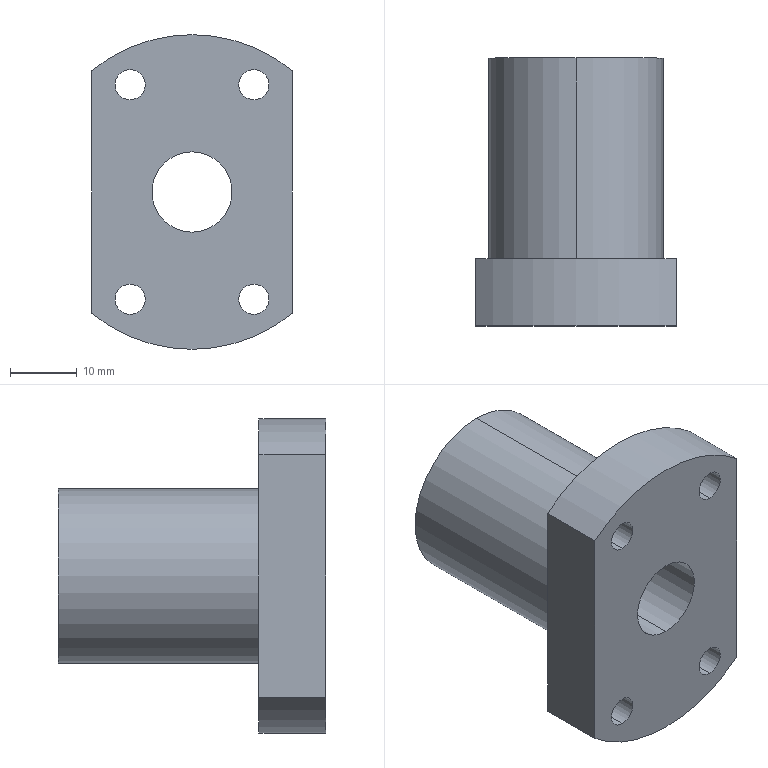Part | NX | features BREP 1 | 1 solid | 20 faces | box 30 x 40 x 47 mm | volume 23841 mm3 | cylinder 15 | plane 5 | commonest cylinder face diameters 4.5 x8 47 x3 12 x2 26 x2
STEP:
#1=CARTESIAN_POINT('',(15.,10.,-18.09));
#2=VERTEX_POINT('',#1);
#3=CARTESIAN_POINT('',(15.,10.,18.09));
#4=VERTEX_POINT('',#3);
#5=CARTESIAN_POINT('',(15.,10.,0.));
#6=DIRECTION('',(0.,0.,1.));
#7=VECTOR('',#6,1000.);
#8=LINE('',#5,#7);
#9=EDGE_CURVE('',#2,#4,#8,.T.);
#10=ORIENTED_EDGE('',*,*,#9,.T.);
#11=CARTESIAN_POINT('',(15.,0.,18.09));
#12=VERTEX_POINT('',#11);
#13=CARTESIAN_POINT('',(15.,40.,18.09));
#14=DIRECTION('',(0.,-1.,0.));
#15=VECTOR('',#14,1000.);
#16=LINE('',#13,#15);
#17=EDGE_CURVE('',#4,#12,#16,.T.);
#18=ORIENTED_EDGE('',*,*,#17,.T.);
#19=CARTESIAN_POINT('',(15.,0.,-18.09));
#20=VERTEX_POINT('',#19);
#21=CARTESIAN_POINT('',(15.,0.,-18.09));
#22=DIRECTION('',(0.,0.,1.));
#23=VECTOR('',#22,1000.);
#24=LINE('',#21,#23);
#25=EDGE_CURVE('',#20,#12,#24,.T.);
#26=ORIENTED_EDGE('',*,*,#25,.F.);
#27=CARTESIAN_POINT('',(15.,40.,-18.09));
#28=DIRECTION('',(0.,-1.,0.));
#29=VECTOR('',#28,1000.);
#30=LINE('',#27,#29);
#31=EDGE_CURVE('',#2,#20,#30,.T.);
#32=ORIENTED_EDGE('',*,*,#31,.F.);
#33=EDGE_LOOP('',(#10,#18,#26,#32));
#34=FACE_BOUND('',#33,.T.);
#35=CARTESIAN_POINT('',(15.,40.,-18.09));
#36=DIRECTION('',(1.,0.,0.));
#37=DIRECTION('',(0.,0.,-1.));
#38=AXIS2_PLACEMENT_3D('',#35,#36,#37);
#39=PLANE('',#38);
#40=ADVANCED_FACE('',(#34),#39,.T.);
#41=CARTESIAN_POINT('',(-15.,10.,18.09));
#42=VERTEX_POINT('',#41);
#43=CARTESIAN_POINT('',(-15.,10.,-18.09));
#44=VERTEX_POINT('',#43);
#45=CARTESIAN_POINT('',(-15.,10.,0.));
#46=DIRECTION('',(0.,0.,-1.));
#47=VECTOR('',#46,1000.);
#48=LINE('',#45,#47);
#49=EDGE_CURVE('',#42,#44,#48,.T.);
#50=ORIENTED_EDGE('',*,*,#49,.T.);
#51=CARTESIAN_POINT('',(-15.,0.,-18.09));
#52=VERTEX_POINT('',#51);
#53=CARTESIAN_POINT('',(-15.,40.,-18.09));
#54=DIRECTION('',(0.,-1.,0.));
#55=VECTOR('',#54,1000.);
#56=LINE('',#53,#55);
#57=EDGE_CURVE('',#44,#52,#56,.T.);
#58=ORIENTED_EDGE('',*,*,#57,.T.);
#59=CARTESIAN_POINT('',(-15.,0.,18.09));
#60=VERTEX_POINT('',#59);
#61=CARTESIAN_POINT('',(-15.,0.,-18.09));
#62=DIRECTION('',(0.,0.,-1.));
#63=VECTOR('',#62,1000.);
#64=LINE('',#61,#63);
#65=EDGE_CURVE('',#60,#52,#64,.T.);
#66=ORIENTED_EDGE('',*,*,#65,.F.);
#67=CARTESIAN_POINT('',(-15.,40.,18.09));
#68=DIRECTION('',(0.,-1.,0.));
#69=VECTOR('',#68,1000.);
#70=LINE('',#67,#69);
#71=EDGE_CURVE('',#42,#60,#70,.T.);
#72=ORIENTED_EDGE('',*,*,#71,.F.);
#73=EDGE_LOOP('',(#50,#58,#66,#72));
#74=FACE_BOUND('',#73,.T.);
#75=CARTESIAN_POINT('',(-15.,40.,-18.09));
#76=DIRECTION('',(-1.,0.,0.));
#77=DIRECTION('',(0.,0.,1.));
#78=AXIS2_PLACEMENT_3D('',#75,#76,#77);
#79=PLANE('',#78);
#80=ADVANCED_FACE('',(#74),#79,.T.);
#81=CARTESIAN_POINT('',(9.25,10.,18.271));
#82=VERTEX_POINT('',#81);
#83=CARTESIAN_POINT('',(9.25,0.,18.271));
#84=VERTEX_POINT('',#83);
#85=CARTESIAN_POINT('',(9.25,40.,18.271));
#86=DIRECTION('',(0.,-1.,0.));
#87=VECTOR('',#86,1000.);
#88=LINE('',#85,#87);
#89=EDGE_CURVE('',#82,#84,#88,.T.);
#90=ORIENTED_EDGE('',*,*,#89,.F.);
#91=CARTESIAN_POINT('',(9.25,10.,13.771));
#92=VERTEX_POINT('',#91);
#93=CARTESIAN_POINT('',(9.25,10.,16.021));
#94=DIRECTION('',(0.,-1.,0.));
#95=DIRECTION('',(0.,0.,-1.));
#96=AXIS2_PLACEMENT_3D('',#93,#94,#95);
#97=CIRCLE('',#96,2.25);
#98=EDGE_CURVE('',#92,#82,#97,.T.);
#99=ORIENTED_EDGE('',*,*,#98,.F.);
#100=CARTESIAN_POINT('',(9.25,0.,13.771));
#101=VERTEX_POINT('',#100);
#102=CARTESIAN_POINT('',(9.25,40.,13.771));
#103=DIRECTION('',(0.,-1.,0.));
#104=VECTOR('',#103,1000.);
#105=LINE('',#102,#104);
#106=EDGE_CURVE('',#92,#101,#105,.T.);
#107=ORIENTED_EDGE('',*,*,#106,.T.);
#108=CARTESIAN_POINT('',(9.25,0.,16.021));
#109=DIRECTION('',(0.,-1.,0.));
#110=DIRECTION('',(0.,0.,1.));
#111=AXIS2_PLACEMENT_3D('',#108,#109,#110);
#112=CIRCLE('',#111,2.25);
#113=EDGE_CURVE('',#101,#84,#112,.T.);
#114=ORIENTED_EDGE('',*,*,#113,.T.);
#115=EDGE_LOOP('',(#90,#99,#107,#114));
#116=FACE_BOUND('',#115,.T.);
#117=CARTESIAN_POINT('',(9.25,40.,16.021));
#118=DIRECTION('',(0.,-1.,0.));
#119=DIRECTION('',(0.,0.,-1.));
#120=AXIS2_PLACEMENT_3D('',#117,#118,#119);
#121=CYLINDRICAL_SURFACE('',#120,2.25);
#122=ADVANCED_FACE('',(#116),#121,.F.);
#123=CARTESIAN_POINT('',(9.25,10.,-13.771));
#124=VERTEX_POINT('',#123);
#125=CARTESIAN_POINT('',(9.25,0.,-13.771));
#126=VERTEX_POINT('',#125);
#127=CARTESIAN_POINT('',(9.25,40.,-13.771));
#128=DIRECTION('',(0.,-1.,0.));
#129=VECTOR('',#128,1000.);
#130=LINE('',#127,#129);
#131=EDGE_CURVE('',#124,#126,#130,.T.);
#132=ORIENTED_EDGE('',*,*,#131,.F.);
#133=CARTESIAN_POINT('',(9.25,10.,-18.271));
#134=VERTEX_POINT('',#133);
#135=CARTESIAN_POINT('',(9.25,10.,-16.021));
#136=DIRECTION('',(0.,-1.,0.));
#137=DIRECTION('',(0.,0.,-1.));
#138=AXIS2_PLACEMENT_3D('',#135,#136,#137);
#139=CIRCLE('',#138,2.25);
#140=EDGE_CURVE('',#134,#124,#139,.T.);
#141=ORIENTED_EDGE('',*,*,#140,.F.);
#142=CARTESIAN_POINT('',(9.25,0.,-18.271));
#143=VERTEX_POINT('',#142);
#144=CARTESIAN_POINT('',(9.25,40.,-18.271));
#145=DIRECTION('',(0.,-1.,0.));
#146=VECTOR('',#145,1000.);
#147=LINE('',#144,#146);
#148=EDGE_CURVE('',#134,#143,#147,.T.);
#149=ORIENTED_EDGE('',*,*,#148,.T.);
#150=CARTESIAN_POINT('',(9.25,0.,-16.021));
#151=DIRECTION('',(0.,-1.,0.));
#152=DIRECTION('',(0.,0.,-1.));
#153=AXIS2_PLACEMENT_3D('',#150,#151,#152);
#154=CIRCLE('',#153,2.25);
#155=EDGE_CURVE('',#143,#126,#154,.T.);
#156=ORIENTED_EDGE('',*,*,#155,.T.);
#157=EDGE_LOOP('',(#132,#141,#149,#156));
#158=FACE_BOUND('',#157,.T.);
#159=CARTESIAN_POINT('',(9.25,40.,-16.021));
#160=DIRECTION('',(0.,-1.,0.));
#161=DIRECTION('',(0.,0.,-1.));
#162=AXIS2_PLACEMENT_3D('',#159,#160,#161);
#163=CYLINDRICAL_SURFACE('',#162,2.25);
#164=ADVANCED_FACE('',(#158),#163,.F.);
#165=CARTESIAN_POINT('',(-9.25,10.,-13.771));
#166=VERTEX_POINT('',#165);
#167=CARTESIAN_POINT('',(-9.25,0.,-13.771));
#168=VERTEX_POINT('',#167);
#169=CARTESIAN_POINT('',(-9.25,40.,-13.771));
#170=DIRECTION('',(0.,-1.,0.));
#171=VECTOR('',#170,1000.);
#172=LINE('',#169,#171);
#173=EDGE_CURVE('',#166,#168,#172,.T.);
#174=ORIENTED_EDGE('',*,*,#173,.F.);
#175=CARTESIAN_POINT('',(-9.25,10.,-18.271));
#176=VERTEX_POINT('',#175);
#177=CARTESIAN_POINT('',(-9.25,10.,-16.021));
#178=DIRECTION('',(0.,-1.,0.));
#179=DIRECTION('',(0.,0.,-1.));
#180=AXIS2_PLACEMENT_3D('',#177,#178,#179);
#181=CIRCLE('',#180,2.25);
#182=EDGE_CURVE('',#176,#166,#181,.T.);
#183=ORIENTED_EDGE('',*,*,#182,.F.);
#184=CARTESIAN_POINT('',(-9.25,0.,-18.271));
#185=VERTEX_POINT('',#184);
#186=CARTESIAN_POINT('',(-9.25,40.,-18.271));
#187=DIRECTION('',(0.,-1.,0.));
#188=VECTOR('',#187,1000.);
#189=LINE('',#186,#188);
#190=EDGE_CURVE('',#176,#185,#189,.T.);
#191=ORIENTED_EDGE('',*,*,#190,.T.);
#192=CARTESIAN_POINT('',(-9.25,0.,-16.021));
#193=DIRECTION('',(0.,-1.,0.));
#194=DIRECTION('',(0.,0.,1.));
#195=AXIS2_PLACEMENT_3D('',#192,#193,#194);
#196=CIRCLE('',#195,2.25);
#197=EDGE_CURVE('',#185,#168,#196,.T.);
#198=ORIENTED_EDGE('',*,*,#197,.T.);
#199=EDGE_LOOP('',(#174,#183,#191,#198));
#200=FACE_BOUND('',#199,.T.);
#201=CARTESIAN_POINT('',(-9.25,40.,-16.021));
#202=DIRECTION('',(0.,-1.,0.));
#203=DIRECTION('',(0.,0.,-1.));
#204=AXIS2_PLACEMENT_3D('',#201,#202,#203);
#205=CYLINDRICAL_SURFACE('',#204,2.25);
#206=ADVANCED_FACE('',(#200),#205,.F.);
#207=CARTESIAN_POINT('',(-9.25,10.,18.271));
#208=VERTEX_POINT('',#207);
#209=CARTESIAN_POINT('',(-9.25,0.,18.271));
#210=VERTEX_POINT('',#209);
#211=CARTESIAN_POINT('',(-9.25,40.,18.271));
#212=DIRECTION('',(0.,-1.,0.));
#213=VECTOR('',#212,1000.);
#214=LINE('',#211,#213);
#215=EDGE_CURVE('',#208,#210,#214,.T.);
#216=ORIENTED_EDGE('',*,*,#215,.F.);
#217=CARTESIAN_POINT('',(-9.25,10.,13.771));
#218=VERTEX_POINT('',#217);
#219=CARTESIAN_POINT('',(-9.25,10.,16.021));
#220=DIRECTION('',(0.,-1.,0.));
#221=DIRECTION('',(0.,0.,-1.));
#222=AXIS2_PLACEMENT_3D('',#219,#220,#221);
#223=CIRCLE('',#222,2.25);
#224=EDGE_CURVE('',#218,#208,#223,.T.);
#225=ORIENTED_EDGE('',*,*,#224,.F.);
#226=CARTESIAN_POINT('',(-9.25,0.,13.771));
#227=VERTEX_POINT('',#226);
#228=CARTESIAN_POINT('',(-9.25,40.,13.771));
#229=DIRECTION('',(0.,-1.,0.));
#230=VECTOR('',#229,1000.);
#231=LINE('',#228,#230);
#232=EDGE_CURVE('',#218,#227,#231,.T.);
#233=ORIENTED_EDGE('',*,*,#232,.T.);
#234=CARTESIAN_POINT('',(-9.25,0.,16.021));
#235=DIRECTION('',(0.,-1.,0.));
#236=DIRECTION('',(0.,0.,-1.));
#237=AXIS2_PLACEMENT_3D('',#234,#235,#236);
#238=CIRCLE('',#237,2.25);
#239=EDGE_CURVE('',#227,#210,#238,.T.);
#240=ORIENTED_EDGE('',*,*,#239,.T.);
#241=EDGE_LOOP('',(#216,#225,#233,#240));
#242=FACE_BOUND('',#241,.T.);
#243=CARTESIAN_POINT('',(-9.25,40.,16.021));
#244=DIRECTION('',(0.,-1.,0.));
#245=DIRECTION('',(0.,0.,-1.));
#246=AXIS2_PLACEMENT_3D('',#243,#244,#245);
#247=CYLINDRICAL_SURFACE('',#246,2.25);
#248=ADVANCED_FACE('',(#242),#247,.F.);
#249=CARTESIAN_POINT('',(0.,40.,-6.));
#250=VERTEX_POINT('',#249);
#251=CARTESIAN_POINT('',(0.,40.,6.));
#252=VERTEX_POINT('',#251);
#253=CARTESIAN_POINT('',(0.,40.,0.));
#254=DIRECTION('',(0.,-1.,0.));
#255=DIRECTION('',(0.,0.,-1.));
#256=AXIS2_PLACEMENT_3D('',#253,#254,#255);
#257=CIRCLE('',#256,6.);
#258=EDGE_CURVE('',#250,#252,#257,.T.);
#259=ORIENTED_EDGE('',*,*,#258,.T.);
#260=CARTESIAN_POINT('',(0.,40.,0.));
#261=DIRECTION('',(0.,-1.,0.));
#262=DIRECTION('',(0.,0.,-1.));
#263=AXIS2_PLACEMENT_3D('',#260,#261,#262);
#264=CIRCLE('',#263,6.);
#265=EDGE_CURVE('',#252,#250,#264,.T.);
#266=ORIENTED_EDGE('',*,*,#265,.T.);
#267=EDGE_LOOP('',(#259,#266));
#268=FACE_BOUND('',#267,.T.);
#269=CARTESIAN_POINT('',(0.,40.,-13.));
#270=VERTEX_POINT('',#269);
#271=CARTESIAN_POINT('',(0.,40.,13.));
#272=VERTEX_POINT('',#271);
#273=CARTESIAN_POINT('',(0.,40.,0.));
#274=DIRECTION('',(0.,-1.,0.));
#275=DIRECTION('',(0.,0.,-1.));
#276=AXIS2_PLACEMENT_3D('',#273,#274,#275);
#277=CIRCLE('',#276,13.);
#278=EDGE_CURVE('',#270,#272,#277,.T.);
#279=ORIENTED_EDGE('',*,*,#278,.F.);
#280=CARTESIAN_POINT('',(0.,40.,0.));
#281=DIRECTION('',(0.,-1.,0.));
#282=DIRECTION('',(0.,0.,-1.));
#283=AXIS2_PLACEMENT_3D('',#280,#281,#282);
#284=CIRCLE('',#283,13.);
#285=EDGE_CURVE('',#272,#270,#284,.T.);
#286=ORIENTED_EDGE('',*,*,#285,.F.);
#287=EDGE_LOOP('',(#279,#286));
#288=FACE_BOUND('',#287,.T.);
#289=CARTESIAN_POINT('',(-13.,40.,0.));
#290=DIRECTION('',(0.,-1.,0.));
#291=DIRECTION('',(0.,0.,-1.));
#292=AXIS2_PLACEMENT_3D('',#289,#290,#291);
#293=PLANE('',#292);
#294=ADVANCED_FACE('',(#268,#288),#293,.F.);
#295=CARTESIAN_POINT('',(0.,10.,13.));
#296=VERTEX_POINT('',#295);
#297=CARTESIAN_POINT('',(0.,0.,13.));
#298=DIRECTION('',(0.,-1.,0.));
#299=VECTOR('',#298,1000.);
#300=LINE('',#297,#299);
#301=EDGE_CURVE('',#272,#296,#300,.T.);
#302=ORIENTED_EDGE('',*,*,#301,.F.);
#303=ORIENTED_EDGE('',*,*,#285,.T.);
#304=CARTESIAN_POINT('',(0.,10.,-13.));
#305=VERTEX_POINT('',#304);
#306=CARTESIAN_POINT('',(0.,0.,-13.));
#307=DIRECTION('',(0.,-1.,0.));
#308=VECTOR('',#307,1000.);
#309=LINE('',#306,#308);
#310=EDGE_CURVE('',#270,#305,#309,.T.);
#311=ORIENTED_EDGE('',*,*,#310,.T.);
#312=CARTESIAN_POINT('',(0.,10.,0.));
#313=DIRECTION('',(0.,-1.,0.));
#314=DIRECTION('',(0.,0.,-1.));
#315=AXIS2_PLACEMENT_3D('',#312,#313,#314);
#316=CIRCLE('',#315,13.);
#317=EDGE_CURVE('',#296,#305,#316,.T.);
#318=ORIENTED_EDGE('',*,*,#317,.F.);
#319=EDGE_LOOP('',(#302,#303,#311,#318));
#320=FACE_BOUND('',#319,.T.);
#321=CARTESIAN_POINT('',(0.,0.,0.));
#322=DIRECTION('',(0.,-1.,0.));
#323=DIRECTION('',(0.,0.,-1.));
#324=AXIS2_PLACEMENT_3D('',#321,#322,#323);
#325=CYLINDRICAL_SURFACE('',#324,13.);
#326=ADVANCED_FACE('',(#320),#325,.T.);
#327=CARTESIAN_POINT('',(0.,0.,6.));
#328=VERTEX_POINT('',#327);
#329=CARTESIAN_POINT('',(0.,0.,6.));
#330=DIRECTION('',(0.,-1.,0.));
#331=VECTOR('',#330,1000.);
#332=LINE('',#329,#331);
#333=EDGE_CURVE('',#252,#328,#332,.T.);
#334=ORIENTED_EDGE('',*,*,#333,.F.);
#335=ORIENTED_EDGE('',*,*,#258,.F.);
#336=CARTESIAN_POINT('',(0.,0.,-6.));
#337=VERTEX_POINT('',#336);
#338=CARTESIAN_POINT('',(0.,0.,-6.));
#339=DIRECTION('',(0.,-1.,0.));
#340=VECTOR('',#339,1000.);
#341=LINE('',#338,#340);
#342=EDGE_CURVE('',#250,#337,#341,.T.);
#343=ORIENTED_EDGE('',*,*,#342,.T.);
#344=CARTESIAN_POINT('',(0.,0.,0.));
#345=DIRECTION('',(0.,-1.,0.));
#346=DIRECTION('',(0.,0.,-1.));
#347=AXIS2_PLACEMENT_3D('',#344,#345,#346);
#348=CIRCLE('',#347,6.);
#349=EDGE_CURVE('',#337,#328,#348,.T.);
#350=ORIENTED_EDGE('',*,*,#349,.T.);
#351=EDGE_LOOP('',(#334,#335,#343,#350));
#352=FACE_BOUND('',#351,.T.);
#353=CARTESIAN_POINT('',(0.,0.,0.));
#354=DIRECTION('',(0.,-1.,0.));
#355=DIRECTION('',(0.,0.,-1.));
#356=AXIS2_PLACEMENT_3D('',#353,#354,#355);
#357=CYLINDRICAL_SURFACE('',#356,6.);
#358=ADVANCED_FACE('',(#352),#357,.F.);
#359=ORIENTED_EDGE('',*,*,#9,.F.);
#360=CARTESIAN_POINT('',(0.,10.,-23.5));
#361=VERTEX_POINT('',#360);
#362=CARTESIAN_POINT('',(0.,10.,0.));
#363=DIRECTION('',(0.,-1.,0.));
#364=DIRECTION('',(0.,0.,-1.));
#365=AXIS2_PLACEMENT_3D('',#362,#363,#364);
#366=CIRCLE('',#365,23.5);
#367=EDGE_CURVE('',#361,#2,#366,.T.);
#368=ORIENTED_EDGE('',*,*,#367,.F.);
#369=CARTESIAN_POINT('',(0.,10.,0.));
#370=DIRECTION('',(0.,-1.,0.));
#371=DIRECTION('',(0.,0.,-1.));
#372=AXIS2_PLACEMENT_3D('',#369,#370,#371);
#373=CIRCLE('',#372,23.5);
#374=EDGE_CURVE('',#44,#361,#373,.T.);
#375=ORIENTED_EDGE('',*,*,#374,.F.);
#376=ORIENTED_EDGE('',*,*,#49,.F.);
#377=CARTESIAN_POINT('',(0.,10.,0.));
#378=DIRECTION('',(0.,-1.,0.));
#379=DIRECTION('',(0.,0.,-1.));
#380=AXIS2_PLACEMENT_3D('',#377,#378,#379);
#381=CIRCLE('',#380,23.5);
#382=EDGE_CURVE('',#4,#42,#381,.T.);
#383=ORIENTED_EDGE('',*,*,#382,.F.);
#384=EDGE_LOOP('',(#359,#368,#375,#376,#383));
#385=FACE_BOUND('',#384,.T.);
#386=CARTESIAN_POINT('',(0.,10.,0.));
#387=DIRECTION('',(0.,-1.,0.));
#388=DIRECTION('',(0.,0.,-1.));
#389=AXIS2_PLACEMENT_3D('',#386,#387,#388);
#390=CIRCLE('',#389,13.);
#391=EDGE_CURVE('',#305,#296,#390,.T.);
#392=ORIENTED_EDGE('',*,*,#391,.T.);
#393=ORIENTED_EDGE('',*,*,#317,.T.);
#394=EDGE_LOOP('',(#392,#393));
#395=FACE_BOUND('',#394,.T.);
#396=ORIENTED_EDGE('',*,*,#224,.T.);
#397=CARTESIAN_POINT('',(-9.25,10.,16.021));
#398=DIRECTION('',(0.,-1.,0.));
#399=DIRECTION('',(0.,0.,-1.));
#400=AXIS2_PLACEMENT_3D('',#397,#398,#399);
#401=CIRCLE('',#400,2.25);
#402=EDGE_CURVE('',#208,#218,#401,.T.);
#403=ORIENTED_EDGE('',*,*,#402,.T.);
#404=EDGE_LOOP('',(#396,#403));
#405=FACE_BOUND('',#404,.T.);
#406=ORIENTED_EDGE('',*,*,#182,.T.);
#407=CARTESIAN_POINT('',(-9.25,10.,-16.021));
#408=DIRECTION('',(0.,-1.,0.));
#409=DIRECTION('',(0.,0.,-1.));
#410=AXIS2_PLACEMENT_3D('',#407,#408,#409);
#411=CIRCLE('',#410,2.25);
#412=EDGE_CURVE('',#166,#176,#411,.T.);
#413=ORIENTED_EDGE('',*,*,#412,.T.);
#414=EDGE_LOOP('',(#406,#413));
#415=FACE_BOUND('',#414,.T.);
#416=ORIENTED_EDGE('',*,*,#140,.T.);
#417=CARTESIAN_POINT('',(9.25,10.,-16.021));
#418=DIRECTION('',(0.,-1.,0.));
#419=DIRECTION('',(0.,0.,-1.));
#420=AXIS2_PLACEMENT_3D('',#417,#418,#419);
#421=CIRCLE('',#420,2.25);
#422=EDGE_CURVE('',#124,#134,#421,.T.);
#423=ORIENTED_EDGE('',*,*,#422,.T.);
#424=EDGE_LOOP('',(#416,#423));
#425=FACE_BOUND('',#424,.T.);
#426=ORIENTED_EDGE('',*,*,#98,.T.);
#427=CARTESIAN_POINT('',(9.25,10.,16.021));
#428=DIRECTION('',(0.,-1.,0.));
#429=DIRECTION('',(0.,0.,-1.));
#430=AXIS2_PLACEMENT_3D('',#427,#428,#429);
#431=CIRCLE('',#430,2.25);
#432=EDGE_CURVE('',#82,#92,#431,.T.);
#433=ORIENTED_EDGE('',*,*,#432,.T.);
#434=EDGE_LOOP('',(#426,#433));
#435=FACE_BOUND('',#434,.T.);
#436=CARTESIAN_POINT('',(-23.5,10.,0.));
#437=DIRECTION('',(0.,-1.,0.));
#438=DIRECTION('',(0.,0.,-1.));
#439=AXIS2_PLACEMENT_3D('',#436,#437,#438);
#440=PLANE('',#439);
#441=ADVANCED_FACE('',(#385,#395,#405,#415,#425,#435),#440,.F.);
#442=ORIENTED_EDGE('',*,*,#17,.F.);
#443=ORIENTED_EDGE('',*,*,#382,.T.);
#444=ORIENTED_EDGE('',*,*,#71,.T.);
#445=CARTESIAN_POINT('',(0.,0.,0.));
#446=DIRECTION('',(0.,-1.,0.));
#447=DIRECTION('',(0.,0.,-1.));
#448=AXIS2_PLACEMENT_3D('',#445,#446,#447);
#449=CIRCLE('',#448,23.5);
#450=EDGE_CURVE('',#12,#60,#449,.T.);
#451=ORIENTED_EDGE('',*,*,#450,.F.);
#452=EDGE_LOOP('',(#442,#443,#444,#451));
#453=FACE_BOUND('',#452,.T.);
#454=CARTESIAN_POINT('',(0.,0.,0.));
#455=DIRECTION('',(0.,-1.,0.));
#456=DIRECTION('',(0.,0.,-1.));
#457=AXIS2_PLACEMENT_3D('',#454,#455,#456);
#458=CYLINDRICAL_SURFACE('',#457,23.5);
#459=ADVANCED_FACE('',(#453),#458,.T.);
#460=CARTESIAN_POINT('',(0.,0.,-23.5));
#461=VERTEX_POINT('',#460);
#462=CARTESIAN_POINT('',(0.,0.,-23.5));
#463=DIRECTION('',(0.,-1.,0.));
#464=VECTOR('',#463,1000.);
#465=LINE('',#462,#464);
#466=EDGE_CURVE('',#361,#461,#465,.T.);
#467=ORIENTED_EDGE('',*,*,#466,.F.);
#468=ORIENTED_EDGE('',*,*,#367,.T.);
#469=ORIENTED_EDGE('',*,*,#31,.T.);
#470=CARTESIAN_POINT('',(0.,0.,0.));
#471=DIRECTION('',(0.,-1.,0.));
#472=DIRECTION('',(0.,0.,-1.));
#473=AXIS2_PLACEMENT_3D('',#470,#471,#472);
#474=CIRCLE('',#473,23.5);
#475=EDGE_CURVE('',#461,#20,#474,.T.);
#476=ORIENTED_EDGE('',*,*,#475,.F.);
#477=EDGE_LOOP('',(#467,#468,#469,#476));
#478=FACE_BOUND('',#477,.T.);
#479=CARTESIAN_POINT('',(0.,0.,0.));
#480=DIRECTION('',(0.,-1.,0.));
#481=DIRECTION('',(0.,0.,-1.));
#482=AXIS2_PLACEMENT_3D('',#479,#480,#481);
#483=CYLINDRICAL_SURFACE('',#482,23.5);
#484=ADVANCED_FACE('',(#478),#483,.T.);
#485=ORIENTED_EDGE('',*,*,#25,.T.);
#486=ORIENTED_EDGE('',*,*,#450,.T.);
#487=ORIENTED_EDGE('',*,*,#65,.T.);
#488=CARTESIAN_POINT('',(0.,0.,0.));
#489=DIRECTION('',(0.,-1.,0.));
#490=DIRECTION('',(0.,0.,-1.));
#491=AXIS2_PLACEMENT_3D('',#488,#489,#490);
#492=CIRCLE('',#491,23.5);
#493=EDGE_CURVE('',#52,#461,#492,.T.);
#494=ORIENTED_EDGE('',*,*,#493,.T.);
#495=ORIENTED_EDGE('',*,*,#475,.T.);
#496=EDGE_LOOP('',(#485,#486,#487,#494,#495));
#497=FACE_BOUND('',#496,.T.);
#498=ORIENTED_EDGE('',*,*,#349,.F.);
#499=CARTESIAN_POINT('',(0.,0.,0.));
#500=DIRECTION('',(0.,-1.,0.));
#501=DIRECTION('',(0.,0.,-1.));
#502=AXIS2_PLACEMENT_3D('',#499,#500,#501);
#503=CIRCLE('',#502,6.);
#504=EDGE_CURVE('',#328,#337,#503,.T.);
#505=ORIENTED_EDGE('',*,*,#504,.F.);
#506=EDGE_LOOP('',(#498,#505));
#507=FACE_BOUND('',#506,.T.);
#508=ORIENTED_EDGE('',*,*,#239,.F.);
#509=CARTESIAN_POINT('',(-9.25,0.,16.021));
#510=DIRECTION('',(0.,-1.,0.));
#511=DIRECTION('',(0.,0.,-1.));
#512=AXIS2_PLACEMENT_3D('',#509,#510,#511);
#513=CIRCLE('',#512,2.25);
#514=EDGE_CURVE('',#210,#227,#513,.T.);
#515=ORIENTED_EDGE('',*,*,#514,.F.);
#516=EDGE_LOOP('',(#508,#515));
#517=FACE_BOUND('',#516,.T.);
#518=ORIENTED_EDGE('',*,*,#197,.F.);
#519=CARTESIAN_POINT('',(-9.25,0.,-16.021));
#520=DIRECTION('',(0.,-1.,0.));
#521=DIRECTION('',(0.,0.,1.));
#522=AXIS2_PLACEMENT_3D('',#519,#520,#521);
#523=CIRCLE('',#522,2.25);
#524=EDGE_CURVE('',#168,#185,#523,.T.);
#525=ORIENTED_EDGE('',*,*,#524,.F.);
#526=EDGE_LOOP('',(#518,#525));
#527=FACE_BOUND('',#526,.T.);
#528=ORIENTED_EDGE('',*,*,#155,.F.);
#529=CARTESIAN_POINT('',(9.25,0.,-16.021));
#530=DIRECTION('',(0.,-1.,0.));
#531=DIRECTION('',(0.,0.,-1.));
#532=AXIS2_PLACEMENT_3D('',#529,#530,#531);
#533=CIRCLE('',#532,2.25);
#534=EDGE_CURVE('',#126,#143,#533,.T.);
#535=ORIENTED_EDGE('',*,*,#534,.F.);
#536=EDGE_LOOP('',(#528,#535));
#537=FACE_BOUND('',#536,.T.);
#538=ORIENTED_EDGE('',*,*,#113,.F.);
#539=CARTESIAN_POINT('',(9.25,0.,16.021));
#540=DIRECTION('',(0.,-1.,0.));
#541=DIRECTION('',(0.,0.,1.));
#542=AXIS2_PLACEMENT_3D('',#539,#540,#541);
#543=CIRCLE('',#542,2.25);
#544=EDGE_CURVE('',#84,#101,#543,.T.);
#545=ORIENTED_EDGE('',*,*,#544,.F.);
#546=EDGE_LOOP('',(#538,#545));
#547=FACE_BOUND('',#546,.T.);
#548=CARTESIAN_POINT('',(-6.,0.,0.));
#549=DIRECTION('',(0.,1.,0.));
#550=DIRECTION('',(0.,0.,1.));
#551=AXIS2_PLACEMENT_3D('',#548,#549,#550);
#552=PLANE('',#551);
#553=ADVANCED_FACE('',(#497,#507,#517,#527,#537,#547),#552,.F.);
#554=ORIENTED_EDGE('',*,*,#374,.T.);
#555=ORIENTED_EDGE('',*,*,#466,.T.);
#556=ORIENTED_EDGE('',*,*,#493,.F.);
#557=ORIENTED_EDGE('',*,*,#57,.F.);
#558=EDGE_LOOP('',(#554,#555,#556,#557));
#559=FACE_BOUND('',#558,.T.);
#560=CARTESIAN_POINT('',(0.,0.,0.));
#561=DIRECTION('',(0.,-1.,0.));
#562=DIRECTION('',(0.,0.,-1.));
#563=AXIS2_PLACEMENT_3D('',#560,#561,#562);
#564=CYLINDRICAL_SURFACE('',#563,23.5);
#565=ADVANCED_FACE('',(#559),#564,.T.);
#566=ORIENTED_EDGE('',*,*,#265,.F.);
#567=ORIENTED_EDGE('',*,*,#333,.T.);
#568=ORIENTED_EDGE('',*,*,#504,.T.);
#569=ORIENTED_EDGE('',*,*,#342,.F.);
#570=EDGE_LOOP('',(#566,#567,#568,#569));
#571=FACE_BOUND('',#570,.T.);
#572=CARTESIAN_POINT('',(0.,0.,0.));
#573=DIRECTION('',(0.,-1.,0.));
#574=DIRECTION('',(0.,0.,-1.));
#575=AXIS2_PLACEMENT_3D('',#572,#573,#574);
#576=CYLINDRICAL_SURFACE('',#575,6.);
#577=ADVANCED_FACE('',(#571),#576,.F.);
#578=ORIENTED_EDGE('',*,*,#278,.T.);
#579=ORIENTED_EDGE('',*,*,#301,.T.);
#580=ORIENTED_EDGE('',*,*,#391,.F.);
#581=ORIENTED_EDGE('',*,*,#310,.F.);
#582=EDGE_LOOP('',(#578,#579,#580,#581));
#583=FACE_BOUND('',#582,.T.);
#584=CARTESIAN_POINT('',(0.,0.,0.));
#585=DIRECTION('',(0.,-1.,0.));
#586=DIRECTION('',(0.,0.,-1.));
#587=AXIS2_PLACEMENT_3D('',#584,#585,#586);
#588=CYLINDRICAL_SURFACE('',#587,13.);
#589=ADVANCED_FACE('',(#583),#588,.T.);
#590=ORIENTED_EDGE('',*,*,#402,.F.);
#591=ORIENTED_EDGE('',*,*,#215,.T.);
#592=ORIENTED_EDGE('',*,*,#514,.T.);
#593=ORIENTED_EDGE('',*,*,#232,.F.);
#594=EDGE_LOOP('',(#590,#591,#592,#593));
#595=FACE_BOUND('',#594,.T.);
#596=CARTESIAN_POINT('',(-9.25,40.,16.021));
#597=DIRECTION('',(0.,-1.,0.));
#598=DIRECTION('',(0.,0.,-1.));
#599=AXIS2_PLACEMENT_3D('',#596,#597,#598);
#600=CYLINDRICAL_SURFACE('',#599,2.25);
#601=ADVANCED_FACE('',(#595),#600,.F.);
#602=ORIENTED_EDGE('',*,*,#412,.F.);
#603=ORIENTED_EDGE('',*,*,#173,.T.);
#604=ORIENTED_EDGE('',*,*,#524,.T.);
#605=ORIENTED_EDGE('',*,*,#190,.F.);
#606=EDGE_LOOP('',(#602,#603,#604,#605));
#607=FACE_BOUND('',#606,.T.);
#608=CARTESIAN_POINT('',(-9.25,40.,-16.021));
#609=DIRECTION('',(0.,-1.,0.));
#610=DIRECTION('',(0.,0.,-1.));
#611=AXIS2_PLACEMENT_3D('',#608,#609,#610);
#612=CYLINDRICAL_SURFACE('',#611,2.25);
#613=ADVANCED_FACE('',(#607),#612,.F.);
#614=ORIENTED_EDGE('',*,*,#422,.F.);
#615=ORIENTED_EDGE('',*,*,#131,.T.);
#616=ORIENTED_EDGE('',*,*,#534,.T.);
#617=ORIENTED_EDGE('',*,*,#148,.F.);
#618=EDGE_LOOP('',(#614,#615,#616,#617));
#619=FACE_BOUND('',#618,.T.);
#620=CARTESIAN_POINT('',(9.25,40.,-16.021));
#621=DIRECTION('',(0.,-1.,0.));
#622=DIRECTION('',(0.,0.,-1.));
#623=AXIS2_PLACEMENT_3D('',#620,#621,#622);
#624=CYLINDRICAL_SURFACE('',#623,2.25);
#625=ADVANCED_FACE('',(#619),#624,.F.);
#626=ORIENTED_EDGE('',*,*,#432,.F.);
#627=ORIENTED_EDGE('',*,*,#89,.T.);
#628=ORIENTED_EDGE('',*,*,#544,.T.);
#629=ORIENTED_EDGE('',*,*,#106,.F.);
#630=EDGE_LOOP('',(#626,#627,#628,#629));
#631=FACE_BOUND('',#630,.T.);
#632=CARTESIAN_POINT('',(9.25,40.,16.021));
#633=DIRECTION('',(0.,-1.,0.));
#634=DIRECTION('',(0.,0.,-1.));
#635=AXIS2_PLACEMENT_3D('',#632,#633,#634);
#636=CYLINDRICAL_SURFACE('',#635,2.25);
#637=ADVANCED_FACE('',(#631),#636,.F.);
#638=CLOSED_SHELL('',(#40,#80,#122,#164,#206,#248,#294,#326,#358,#441,#459,#484,#553,#565,#577,#589,#601,#613,#625,#637));
#639=MANIFOLD_SOLID_BREP('',#638);
#640=(LENGTH_UNIT()NAMED_UNIT(*)SI_UNIT(.MILLI.,.METRE.));
#641=UNCERTAINTY_MEASURE_WITH_UNIT(LENGTH_MEASURE(0.00001),#640,'','');
#642=(NAMED_UNIT(*)PLANE_ANGLE_UNIT()SI_UNIT($,.RADIAN.));
#643=(NAMED_UNIT(*)SI_UNIT($,.STERADIAN.)SOLID_ANGLE_UNIT());
#644=(GEOMETRIC_REPRESENTATION_CONTEXT(3)GLOBAL_UNCERTAINTY_ASSIGNED_CONTEXT((#641))GLOBAL_UNIT_ASSIGNED_CONTEXT((#640,#642,#643))REPRESENTATION_CONTEXT('',''));
#645=ADVANCED_BREP_SHAPE_REPRESENTATION('',(#639),#644);